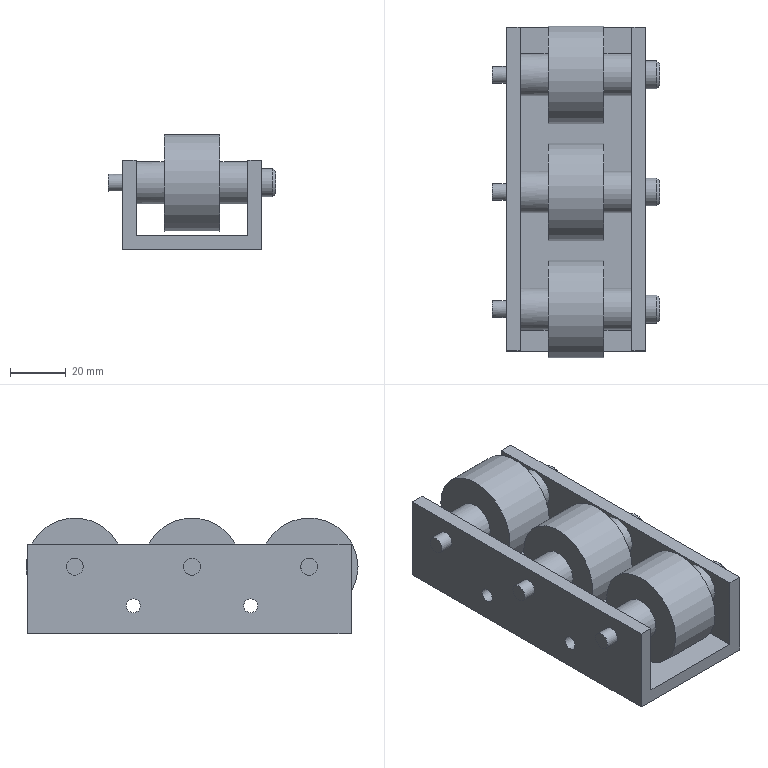Part | NX | features solid 2 | 1 solid | 44 faces | box 60 x 119 x 41.5 mm | volume 129815 mm3 | plane 22 | cylinder 19 | cone 3 | commonest cylinder face diameters 15 x6 5 x4 6 x3 10 x3 35 x3
STEP:
#1=CARTESIAN_POINT('',(215.,191.,-18.));
#2=VERTEX_POINT('',#1);
#3=CARTESIAN_POINT('',(215.,191.,-50.));
#4=VERTEX_POINT('',#3);
#5=CARTESIAN_POINT('',(215.,191.,-18.));
#6=DIRECTION('',(0.,0.,-1.));
#7=VECTOR('',#6,1000.);
#8=LINE('',#5,#7);
#9=EDGE_CURVE('',#2,#4,#8,.T.);
#10=ORIENTED_EDGE('',*,*,#9,.T.);
#11=CARTESIAN_POINT('',(165.,191.,-50.));
#12=VERTEX_POINT('',#11);
#13=CARTESIAN_POINT('',(215.,191.,-50.));
#14=DIRECTION('',(-1.,0.,0.));
#15=VECTOR('',#14,1000.);
#16=LINE('',#13,#15);
#17=EDGE_CURVE('',#4,#12,#16,.T.);
#18=ORIENTED_EDGE('',*,*,#17,.T.);
#19=CARTESIAN_POINT('',(165.,191.,-18.));
#20=VERTEX_POINT('',#19);
#21=CARTESIAN_POINT('',(165.,191.,-50.));
#22=DIRECTION('',(0.,0.,1.));
#23=VECTOR('',#22,1000.);
#24=LINE('',#21,#23);
#25=EDGE_CURVE('',#12,#20,#24,.T.);
#26=ORIENTED_EDGE('',*,*,#25,.T.);
#27=CARTESIAN_POINT('',(170.,191.,-18.));
#28=VERTEX_POINT('',#27);
#29=CARTESIAN_POINT('',(165.,191.,-18.));
#30=DIRECTION('',(1.,0.,0.));
#31=VECTOR('',#30,1000.);
#32=LINE('',#29,#31);
#33=EDGE_CURVE('',#20,#28,#32,.T.);
#34=ORIENTED_EDGE('',*,*,#33,.T.);
#35=CARTESIAN_POINT('',(170.,191.,-45.));
#36=VERTEX_POINT('',#35);
#37=CARTESIAN_POINT('',(170.,191.,-50.));
#38=DIRECTION('',(0.,0.,1.));
#39=VECTOR('',#38,1000.);
#40=LINE('',#37,#39);
#41=EDGE_CURVE('',#36,#28,#40,.T.);
#42=ORIENTED_EDGE('',*,*,#41,.F.);
#43=CARTESIAN_POINT('',(210.,191.,-45.));
#44=VERTEX_POINT('',#43);
#45=CARTESIAN_POINT('',(215.,191.,-45.));
#46=DIRECTION('',(-1.,0.,0.));
#47=VECTOR('',#46,1000.);
#48=LINE('',#45,#47);
#49=EDGE_CURVE('',#44,#36,#48,.T.);
#50=ORIENTED_EDGE('',*,*,#49,.F.);
#51=CARTESIAN_POINT('',(210.,191.,-18.));
#52=VERTEX_POINT('',#51);
#53=CARTESIAN_POINT('',(210.,191.,-18.));
#54=DIRECTION('',(0.,0.,-1.));
#55=VECTOR('',#54,1000.);
#56=LINE('',#53,#55);
#57=EDGE_CURVE('',#52,#44,#56,.T.);
#58=ORIENTED_EDGE('',*,*,#57,.F.);
#59=CARTESIAN_POINT('',(215.,191.,-18.));
#60=DIRECTION('',(-1.,0.,0.));
#61=VECTOR('',#60,1000.);
#62=LINE('',#59,#61);
#63=EDGE_CURVE('',#52,#2,#62,.F.);
#64=ORIENTED_EDGE('',*,*,#63,.T.);
#65=EDGE_LOOP('',(#10,#18,#26,#34,#42,#50,#58,#64));
#66=FACE_BOUND('',#65,.T.);
#67=CARTESIAN_POINT('',(190.,191.,-34.));
#68=DIRECTION('',(0.,1.,0.));
#69=DIRECTION('',(0.,0.,1.));
#70=AXIS2_PLACEMENT_3D('',#67,#68,#69);
#71=PLANE('',#70);
#72=ADVANCED_FACE('',(#66),#71,.T.);
#73=CARTESIAN_POINT('',(220.,174.,-22.));
#74=VERTEX_POINT('',#73);
#75=CARTESIAN_POINT('',(220.,174.,-26.));
#76=DIRECTION('',(1.,0.,0.));
#77=DIRECTION('',(0.,0.,1.));
#78=AXIS2_PLACEMENT_3D('',#75,#76,#77);
#79=CIRCLE('',#78,4.);
#80=EDGE_CURVE('',#74,#74,#79,.F.);
#81=ORIENTED_EDGE('',*,*,#80,.F.);
#82=EDGE_LOOP('',(#81));
#83=FACE_BOUND('',#82,.T.);
#84=CARTESIAN_POINT('',(220.,174.,-26.));
#85=DIRECTION('',(-1.,0.,0.));
#86=DIRECTION('',(0.,0.,1.));
#87=AXIS2_PLACEMENT_3D('',#84,#85,#86);
#88=PLANE('',#87);
#89=ADVANCED_FACE('',(#83),#88,.F.);
#90=CARTESIAN_POINT('',(220.,132.,-22.));
#91=VERTEX_POINT('',#90);
#92=CARTESIAN_POINT('',(220.,132.,-26.));
#93=DIRECTION('',(1.,0.,0.));
#94=DIRECTION('',(0.,0.,1.));
#95=AXIS2_PLACEMENT_3D('',#92,#93,#94);
#96=CIRCLE('',#95,4.);
#97=EDGE_CURVE('',#91,#91,#96,.F.);
#98=ORIENTED_EDGE('',*,*,#97,.F.);
#99=EDGE_LOOP('',(#98));
#100=FACE_BOUND('',#99,.T.);
#101=CARTESIAN_POINT('',(220.,132.,-26.));
#102=DIRECTION('',(-1.,0.,0.));
#103=DIRECTION('',(0.,0.,1.));
#104=AXIS2_PLACEMENT_3D('',#101,#102,#103);
#105=PLANE('',#104);
#106=ADVANCED_FACE('',(#100),#105,.F.);
#107=CARTESIAN_POINT('',(220.,90.,-22.));
#108=VERTEX_POINT('',#107);
#109=CARTESIAN_POINT('',(220.,90.,-26.));
#110=DIRECTION('',(1.,0.,0.));
#111=DIRECTION('',(0.,0.,1.));
#112=AXIS2_PLACEMENT_3D('',#109,#110,#111);
#113=CIRCLE('',#112,4.);
#114=EDGE_CURVE('',#108,#108,#113,.F.);
#115=ORIENTED_EDGE('',*,*,#114,.F.);
#116=EDGE_LOOP('',(#115));
#117=FACE_BOUND('',#116,.T.);
#118=CARTESIAN_POINT('',(220.,90.,-26.));
#119=DIRECTION('',(-1.,0.,0.));
#120=DIRECTION('',(0.,0.,1.));
#121=AXIS2_PLACEMENT_3D('',#118,#119,#120);
#122=PLANE('',#121);
#123=ADVANCED_FACE('',(#117),#122,.F.);
#124=CARTESIAN_POINT('',(180.,114.5,-26.));
#125=VERTEX_POINT('',#124);
#126=CARTESIAN_POINT('',(180.,132.,-26.));
#127=DIRECTION('',(1.,0.,0.));
#128=DIRECTION('',(0.,-1.,0.));
#129=AXIS2_PLACEMENT_3D('',#126,#127,#128);
#130=CIRCLE('',#129,17.5);
#131=EDGE_CURVE('',#125,#125,#130,.T.);
#132=ORIENTED_EDGE('',*,*,#131,.T.);
#133=EDGE_LOOP('',(#132));
#134=FACE_BOUND('',#133,.T.);
#135=CARTESIAN_POINT('',(200.,114.5,-26.));
#136=VERTEX_POINT('',#135);
#137=CARTESIAN_POINT('',(200.,132.,-26.));
#138=DIRECTION('',(1.,0.,0.));
#139=DIRECTION('',(0.,-1.,0.));
#140=AXIS2_PLACEMENT_3D('',#137,#138,#139);
#141=CIRCLE('',#140,17.5);
#142=EDGE_CURVE('',#136,#136,#141,.T.);
#143=ORIENTED_EDGE('',*,*,#142,.F.);
#144=EDGE_LOOP('',(#143));
#145=FACE_BOUND('',#144,.T.);
#146=CARTESIAN_POINT('',(180.,132.,-26.));
#147=DIRECTION('',(1.,0.,0.));
#148=DIRECTION('',(0.,0.,-1.));
#149=AXIS2_PLACEMENT_3D('',#146,#147,#148);
#150=CYLINDRICAL_SURFACE('',#149,17.5);
#151=ADVANCED_FACE('',(#134,#145),#150,.T.);
#152=CARTESIAN_POINT('',(200.,72.5,-26.));
#153=VERTEX_POINT('',#152);
#154=CARTESIAN_POINT('',(200.,90.,-26.));
#155=DIRECTION('',(1.,0.,0.));
#156=DIRECTION('',(0.,-1.,0.));
#157=AXIS2_PLACEMENT_3D('',#154,#155,#156);
#158=CIRCLE('',#157,17.5);
#159=EDGE_CURVE('',#153,#153,#158,.T.);
#160=ORIENTED_EDGE('',*,*,#159,.F.);
#161=EDGE_LOOP('',(#160));
#162=FACE_BOUND('',#161,.T.);
#163=CARTESIAN_POINT('',(180.,72.5,-26.));
#164=VERTEX_POINT('',#163);
#165=CARTESIAN_POINT('',(180.,90.,-26.));
#166=DIRECTION('',(1.,0.,0.));
#167=DIRECTION('',(0.,-1.,0.));
#168=AXIS2_PLACEMENT_3D('',#165,#166,#167);
#169=CIRCLE('',#168,17.5);
#170=EDGE_CURVE('',#164,#164,#169,.T.);
#171=ORIENTED_EDGE('',*,*,#170,.T.);
#172=EDGE_LOOP('',(#171));
#173=FACE_BOUND('',#172,.T.);
#174=CARTESIAN_POINT('',(180.,90.,-26.));
#175=DIRECTION('',(1.,0.,0.));
#176=DIRECTION('',(0.,0.,-1.));
#177=AXIS2_PLACEMENT_3D('',#174,#175,#176);
#178=CYLINDRICAL_SURFACE('',#177,17.5);
#179=ADVANCED_FACE('',(#162,#173),#178,.T.);
#180=ORIENTED_EDGE('',*,*,#80,.T.);
#181=EDGE_LOOP('',(#180));
#182=FACE_BOUND('',#181,.T.);
#183=CARTESIAN_POINT('',(219.,174.,-21.));
#184=VERTEX_POINT('',#183);
#185=CARTESIAN_POINT('',(219.,174.,-26.));
#186=DIRECTION('',(1.,0.,0.));
#187=DIRECTION('',(0.,0.,1.));
#188=AXIS2_PLACEMENT_3D('',#185,#186,#187);
#189=CIRCLE('',#188,5.);
#190=EDGE_CURVE('',#184,#184,#189,.T.);
#191=ORIENTED_EDGE('',*,*,#190,.T.);
#192=EDGE_LOOP('',(#191));
#193=FACE_BOUND('',#192,.T.);
#194=CARTESIAN_POINT('',(219.,174.,-26.));
#195=DIRECTION('',(-1.,0.,0.));
#196=DIRECTION('',(0.,0.,1.));
#197=AXIS2_PLACEMENT_3D('',#194,#195,#196);
#198=CONICAL_SURFACE('',#197,5.,0.7854);
#199=ADVANCED_FACE('',(#182,#193),#198,.T.);
#200=ORIENTED_EDGE('',*,*,#97,.T.);
#201=EDGE_LOOP('',(#200));
#202=FACE_BOUND('',#201,.T.);
#203=CARTESIAN_POINT('',(219.,132.,-21.));
#204=VERTEX_POINT('',#203);
#205=CARTESIAN_POINT('',(219.,132.,-26.));
#206=DIRECTION('',(1.,0.,0.));
#207=DIRECTION('',(0.,0.,1.));
#208=AXIS2_PLACEMENT_3D('',#205,#206,#207);
#209=CIRCLE('',#208,5.);
#210=EDGE_CURVE('',#204,#204,#209,.T.);
#211=ORIENTED_EDGE('',*,*,#210,.T.);
#212=EDGE_LOOP('',(#211));
#213=FACE_BOUND('',#212,.T.);
#214=CARTESIAN_POINT('',(219.,132.,-26.));
#215=DIRECTION('',(-1.,0.,0.));
#216=DIRECTION('',(0.,0.,1.));
#217=AXIS2_PLACEMENT_3D('',#214,#215,#216);
#218=CONICAL_SURFACE('',#217,5.,0.7854);
#219=ADVANCED_FACE('',(#202,#213),#218,.T.);
#220=ORIENTED_EDGE('',*,*,#114,.T.);
#221=EDGE_LOOP('',(#220));
#222=FACE_BOUND('',#221,.T.);
#223=CARTESIAN_POINT('',(219.,90.,-21.));
#224=VERTEX_POINT('',#223);
#225=CARTESIAN_POINT('',(219.,90.,-26.));
#226=DIRECTION('',(1.,0.,0.));
#227=DIRECTION('',(0.,0.,1.));
#228=AXIS2_PLACEMENT_3D('',#225,#226,#227);
#229=CIRCLE('',#228,5.);
#230=EDGE_CURVE('',#224,#224,#229,.T.);
#231=ORIENTED_EDGE('',*,*,#230,.T.);
#232=EDGE_LOOP('',(#231));
#233=FACE_BOUND('',#232,.T.);
#234=CARTESIAN_POINT('',(219.,90.,-26.));
#235=DIRECTION('',(-1.,0.,0.));
#236=DIRECTION('',(0.,0.,1.));
#237=AXIS2_PLACEMENT_3D('',#234,#235,#236);
#238=CONICAL_SURFACE('',#237,5.,0.7854);
#239=ADVANCED_FACE('',(#222,#233),#238,.T.);
#240=CARTESIAN_POINT('',(160.,129.,-26.));
#241=VERTEX_POINT('',#240);
#242=CARTESIAN_POINT('',(160.,132.,-26.));
#243=DIRECTION('',(1.,0.,0.));
#244=DIRECTION('',(0.,-1.,0.));
#245=AXIS2_PLACEMENT_3D('',#242,#243,#244);
#246=CIRCLE('',#245,3.);
#247=EDGE_CURVE('',#241,#241,#246,.T.);
#248=ORIENTED_EDGE('',*,*,#247,.F.);
#249=EDGE_LOOP('',(#248));
#250=FACE_BOUND('',#249,.T.);
#251=CARTESIAN_POINT('',(160.,132.,-26.));
#252=DIRECTION('',(-1.,0.,0.));
#253=DIRECTION('',(0.,0.,1.));
#254=AXIS2_PLACEMENT_3D('',#251,#252,#253);
#255=PLANE('',#254);
#256=ADVANCED_FACE('',(#250),#255,.T.);
#257=CARTESIAN_POINT('',(160.,171.,-26.));
#258=VERTEX_POINT('',#257);
#259=CARTESIAN_POINT('',(160.,174.,-26.));
#260=DIRECTION('',(1.,0.,0.));
#261=DIRECTION('',(0.,-1.,0.));
#262=AXIS2_PLACEMENT_3D('',#259,#260,#261);
#263=CIRCLE('',#262,3.);
#264=EDGE_CURVE('',#258,#258,#263,.T.);
#265=ORIENTED_EDGE('',*,*,#264,.F.);
#266=EDGE_LOOP('',(#265));
#267=FACE_BOUND('',#266,.T.);
#268=CARTESIAN_POINT('',(160.,174.,-26.));
#269=DIRECTION('',(-1.,0.,0.));
#270=DIRECTION('',(0.,0.,1.));
#271=AXIS2_PLACEMENT_3D('',#268,#269,#270);
#272=PLANE('',#271);
#273=ADVANCED_FACE('',(#267),#272,.T.);
#274=CARTESIAN_POINT('',(160.,87.,-26.));
#275=VERTEX_POINT('',#274);
#276=CARTESIAN_POINT('',(160.,90.,-26.));
#277=DIRECTION('',(1.,0.,0.));
#278=DIRECTION('',(0.,-1.,0.));
#279=AXIS2_PLACEMENT_3D('',#276,#277,#278);
#280=CIRCLE('',#279,3.);
#281=EDGE_CURVE('',#275,#275,#280,.T.);
#282=ORIENTED_EDGE('',*,*,#281,.F.);
#283=EDGE_LOOP('',(#282));
#284=FACE_BOUND('',#283,.T.);
#285=CARTESIAN_POINT('',(160.,90.,-26.));
#286=DIRECTION('',(-1.,0.,0.));
#287=DIRECTION('',(0.,0.,1.));
#288=AXIS2_PLACEMENT_3D('',#285,#286,#287);
#289=PLANE('',#288);
#290=ADVANCED_FACE('',(#284),#289,.T.);
#291=CARTESIAN_POINT('',(200.,124.5,-26.));
#292=VERTEX_POINT('',#291);
#293=CARTESIAN_POINT('',(200.,132.,-26.));
#294=DIRECTION('',(1.,0.,0.));
#295=DIRECTION('',(0.,-1.,0.));
#296=AXIS2_PLACEMENT_3D('',#293,#294,#295);
#297=CIRCLE('',#296,7.5);
#298=EDGE_CURVE('',#292,#292,#297,.T.);
#299=ORIENTED_EDGE('',*,*,#298,.F.);
#300=EDGE_LOOP('',(#299));
#301=FACE_BOUND('',#300,.T.);
#302=ORIENTED_EDGE('',*,*,#142,.T.);
#303=EDGE_LOOP('',(#302));
#304=FACE_BOUND('',#303,.T.);
#305=CARTESIAN_POINT('',(200.,132.,-26.));
#306=DIRECTION('',(-1.,0.,0.));
#307=DIRECTION('',(0.,0.,1.));
#308=AXIS2_PLACEMENT_3D('',#305,#306,#307);
#309=PLANE('',#308);
#310=ADVANCED_FACE('',(#301,#304),#309,.F.);
#311=CARTESIAN_POINT('',(200.,82.5,-26.));
#312=VERTEX_POINT('',#311);
#313=CARTESIAN_POINT('',(200.,90.,-26.));
#314=DIRECTION('',(1.,0.,0.));
#315=DIRECTION('',(0.,-1.,0.));
#316=AXIS2_PLACEMENT_3D('',#313,#314,#315);
#317=CIRCLE('',#316,7.5);
#318=EDGE_CURVE('',#312,#312,#317,.T.);
#319=ORIENTED_EDGE('',*,*,#318,.F.);
#320=EDGE_LOOP('',(#319));
#321=FACE_BOUND('',#320,.T.);
#322=ORIENTED_EDGE('',*,*,#159,.T.);
#323=EDGE_LOOP('',(#322));
#324=FACE_BOUND('',#323,.T.);
#325=CARTESIAN_POINT('',(200.,90.,-26.));
#326=DIRECTION('',(-1.,0.,0.));
#327=DIRECTION('',(0.,0.,1.));
#328=AXIS2_PLACEMENT_3D('',#325,#326,#327);
#329=PLANE('',#328);
#330=ADVANCED_FACE('',(#321,#324),#329,.F.);
#331=ORIENTED_EDGE('',*,*,#131,.F.);
#332=EDGE_LOOP('',(#331));
#333=FACE_BOUND('',#332,.T.);
#334=CARTESIAN_POINT('',(180.,124.5,-26.));
#335=VERTEX_POINT('',#334);
#336=CARTESIAN_POINT('',(180.,132.,-26.));
#337=DIRECTION('',(1.,0.,0.));
#338=DIRECTION('',(0.,-1.,0.));
#339=AXIS2_PLACEMENT_3D('',#336,#337,#338);
#340=CIRCLE('',#339,7.5);
#341=EDGE_CURVE('',#335,#335,#340,.T.);
#342=ORIENTED_EDGE('',*,*,#341,.T.);
#343=EDGE_LOOP('',(#342));
#344=FACE_BOUND('',#343,.T.);
#345=CARTESIAN_POINT('',(180.,132.,-26.));
#346=DIRECTION('',(-1.,0.,0.));
#347=DIRECTION('',(0.,0.,1.));
#348=AXIS2_PLACEMENT_3D('',#345,#346,#347);
#349=PLANE('',#348);
#350=ADVANCED_FACE('',(#333,#344),#349,.T.);
#351=CARTESIAN_POINT('',(180.,82.5,-26.));
#352=VERTEX_POINT('',#351);
#353=CARTESIAN_POINT('',(180.,90.,-26.));
#354=DIRECTION('',(1.,0.,0.));
#355=DIRECTION('',(0.,-1.,0.));
#356=AXIS2_PLACEMENT_3D('',#353,#354,#355);
#357=CIRCLE('',#356,7.5);
#358=EDGE_CURVE('',#352,#352,#357,.T.);
#359=ORIENTED_EDGE('',*,*,#358,.T.);
#360=EDGE_LOOP('',(#359));
#361=FACE_BOUND('',#360,.T.);
#362=ORIENTED_EDGE('',*,*,#170,.F.);
#363=EDGE_LOOP('',(#362));
#364=FACE_BOUND('',#363,.T.);
#365=CARTESIAN_POINT('',(180.,90.,-26.));
#366=DIRECTION('',(-1.,0.,0.));
#367=DIRECTION('',(0.,0.,1.));
#368=AXIS2_PLACEMENT_3D('',#365,#366,#367);
#369=PLANE('',#368);
#370=ADVANCED_FACE('',(#361,#364),#369,.T.);
#371=ORIENTED_EDGE('',*,*,#190,.F.);
#372=EDGE_LOOP('',(#371));
#373=FACE_BOUND('',#372,.T.);
#374=CARTESIAN_POINT('',(215.,174.,-31.));
#375=VERTEX_POINT('',#374);
#376=CARTESIAN_POINT('',(215.,174.,-26.));
#377=DIRECTION('',(-1.,0.,0.));
#378=DIRECTION('',(0.,0.,-1.));
#379=AXIS2_PLACEMENT_3D('',#376,#377,#378);
#380=CIRCLE('',#379,5.);
#381=EDGE_CURVE('',#375,#375,#380,.T.);
#382=ORIENTED_EDGE('',*,*,#381,.F.);
#383=EDGE_LOOP('',(#382));
#384=FACE_BOUND('',#383,.T.);
#385=CARTESIAN_POINT('',(220.,174.,-26.));
#386=DIRECTION('',(-1.,0.,0.));
#387=DIRECTION('',(0.,0.,1.));
#388=AXIS2_PLACEMENT_3D('',#385,#386,#387);
#389=CYLINDRICAL_SURFACE('',#388,5.);
#390=ADVANCED_FACE('',(#373,#384),#389,.T.);
#391=ORIENTED_EDGE('',*,*,#210,.F.);
#392=EDGE_LOOP('',(#391));
#393=FACE_BOUND('',#392,.T.);
#394=CARTESIAN_POINT('',(215.,132.,-31.));
#395=VERTEX_POINT('',#394);
#396=CARTESIAN_POINT('',(215.,132.,-26.));
#397=DIRECTION('',(-1.,0.,0.));
#398=DIRECTION('',(0.,0.,-1.));
#399=AXIS2_PLACEMENT_3D('',#396,#397,#398);
#400=CIRCLE('',#399,5.);
#401=EDGE_CURVE('',#395,#395,#400,.T.);
#402=ORIENTED_EDGE('',*,*,#401,.F.);
#403=EDGE_LOOP('',(#402));
#404=FACE_BOUND('',#403,.T.);
#405=CARTESIAN_POINT('',(220.,132.,-26.));
#406=DIRECTION('',(-1.,0.,0.));
#407=DIRECTION('',(0.,0.,1.));
#408=AXIS2_PLACEMENT_3D('',#405,#406,#407);
#409=CYLINDRICAL_SURFACE('',#408,5.);
#410=ADVANCED_FACE('',(#393,#404),#409,.T.);
#411=ORIENTED_EDGE('',*,*,#230,.F.);
#412=EDGE_LOOP('',(#411));
#413=FACE_BOUND('',#412,.T.);
#414=CARTESIAN_POINT('',(215.,90.,-31.));
#415=VERTEX_POINT('',#414);
#416=CARTESIAN_POINT('',(215.,90.,-26.));
#417=DIRECTION('',(-1.,0.,0.));
#418=DIRECTION('',(0.,0.,-1.));
#419=AXIS2_PLACEMENT_3D('',#416,#417,#418);
#420=CIRCLE('',#419,5.);
#421=EDGE_CURVE('',#415,#415,#420,.T.);
#422=ORIENTED_EDGE('',*,*,#421,.F.);
#423=EDGE_LOOP('',(#422));
#424=FACE_BOUND('',#423,.T.);
#425=CARTESIAN_POINT('',(220.,90.,-26.));
#426=DIRECTION('',(-1.,0.,0.));
#427=DIRECTION('',(0.,0.,1.));
#428=AXIS2_PLACEMENT_3D('',#425,#426,#427);
#429=CYLINDRICAL_SURFACE('',#428,5.);
#430=ADVANCED_FACE('',(#413,#424),#429,.T.);
#431=CARTESIAN_POINT('',(165.,132.,-23.));
#432=VERTEX_POINT('',#431);
#433=CARTESIAN_POINT('',(165.,132.,-26.));
#434=DIRECTION('',(1.,0.,0.));
#435=DIRECTION('',(0.,0.,1.));
#436=AXIS2_PLACEMENT_3D('',#433,#434,#435);
#437=CIRCLE('',#436,3.);
#438=EDGE_CURVE('',#432,#432,#437,.F.);
#439=ORIENTED_EDGE('',*,*,#438,.T.);
#440=EDGE_LOOP('',(#439));
#441=FACE_BOUND('',#440,.T.);
#442=ORIENTED_EDGE('',*,*,#247,.T.);
#443=EDGE_LOOP('',(#442));
#444=FACE_BOUND('',#443,.T.);
#445=CARTESIAN_POINT('',(160.,132.,-26.));
#446=DIRECTION('',(1.,0.,0.));
#447=DIRECTION('',(0.,0.,-1.));
#448=AXIS2_PLACEMENT_3D('',#445,#446,#447);
#449=CYLINDRICAL_SURFACE('',#448,3.);
#450=ADVANCED_FACE('',(#441,#444),#449,.T.);
#451=CARTESIAN_POINT('',(165.,174.,-23.));
#452=VERTEX_POINT('',#451);
#453=CARTESIAN_POINT('',(165.,174.,-26.));
#454=DIRECTION('',(1.,0.,0.));
#455=DIRECTION('',(0.,0.,1.));
#456=AXIS2_PLACEMENT_3D('',#453,#454,#455);
#457=CIRCLE('',#456,3.);
#458=EDGE_CURVE('',#452,#452,#457,.F.);
#459=ORIENTED_EDGE('',*,*,#458,.T.);
#460=EDGE_LOOP('',(#459));
#461=FACE_BOUND('',#460,.T.);
#462=ORIENTED_EDGE('',*,*,#264,.T.);
#463=EDGE_LOOP('',(#462));
#464=FACE_BOUND('',#463,.T.);
#465=CARTESIAN_POINT('',(160.,174.,-26.));
#466=DIRECTION('',(1.,0.,0.));
#467=DIRECTION('',(0.,0.,-1.));
#468=AXIS2_PLACEMENT_3D('',#465,#466,#467);
#469=CYLINDRICAL_SURFACE('',#468,3.);
#470=ADVANCED_FACE('',(#461,#464),#469,.T.);
#471=CARTESIAN_POINT('',(165.,90.,-23.));
#472=VERTEX_POINT('',#471);
#473=CARTESIAN_POINT('',(165.,90.,-26.));
#474=DIRECTION('',(1.,0.,0.));
#475=DIRECTION('',(0.,0.,1.));
#476=AXIS2_PLACEMENT_3D('',#473,#474,#475);
#477=CIRCLE('',#476,3.);
#478=EDGE_CURVE('',#472,#472,#477,.F.);
#479=ORIENTED_EDGE('',*,*,#478,.T.);
#480=EDGE_LOOP('',(#479));
#481=FACE_BOUND('',#480,.T.);
#482=ORIENTED_EDGE('',*,*,#281,.T.);
#483=EDGE_LOOP('',(#482));
#484=FACE_BOUND('',#483,.T.);
#485=CARTESIAN_POINT('',(160.,90.,-26.));
#486=DIRECTION('',(1.,0.,0.));
#487=DIRECTION('',(0.,0.,-1.));
#488=AXIS2_PLACEMENT_3D('',#485,#486,#487);
#489=CYLINDRICAL_SURFACE('',#488,3.);
#490=ADVANCED_FACE('',(#481,#484),#489,.T.);
#491=CARTESIAN_POINT('',(215.,111.,-42.5));
#492=VERTEX_POINT('',#491);
#493=CARTESIAN_POINT('',(215.,111.,-40.));
#494=DIRECTION('',(-1.,0.,0.));
#495=DIRECTION('',(0.,0.,-1.));
#496=AXIS2_PLACEMENT_3D('',#493,#494,#495);
#497=CIRCLE('',#496,2.5);
#498=EDGE_CURVE('',#492,#492,#497,.F.);
#499=ORIENTED_EDGE('',*,*,#498,.T.);
#500=EDGE_LOOP('',(#499));
#501=FACE_BOUND('',#500,.T.);
#502=CARTESIAN_POINT('',(210.,111.,-42.5));
#503=VERTEX_POINT('',#502);
#504=CARTESIAN_POINT('',(210.,111.,-40.));
#505=DIRECTION('',(-1.,0.,0.));
#506=DIRECTION('',(0.,0.,-1.));
#507=AXIS2_PLACEMENT_3D('',#504,#505,#506);
#508=CIRCLE('',#507,2.5);
#509=EDGE_CURVE('',#503,#503,#508,.F.);
#510=ORIENTED_EDGE('',*,*,#509,.F.);
#511=EDGE_LOOP('',(#510));
#512=FACE_BOUND('',#511,.T.);
#513=CARTESIAN_POINT('',(160.,111.,-40.));
#514=DIRECTION('',(1.,0.,0.));
#515=DIRECTION('',(0.,0.,-1.));
#516=AXIS2_PLACEMENT_3D('',#513,#514,#515);
#517=CYLINDRICAL_SURFACE('',#516,2.5);
#518=ADVANCED_FACE('',(#501,#512),#517,.F.);
#519=CARTESIAN_POINT('',(210.,124.5,-26.));
#520=VERTEX_POINT('',#519);
#521=CARTESIAN_POINT('',(210.,132.,-26.));
#522=DIRECTION('',(1.,0.,0.));
#523=DIRECTION('',(0.,-1.,0.));
#524=AXIS2_PLACEMENT_3D('',#521,#522,#523);
#525=CIRCLE('',#524,7.5);
#526=EDGE_CURVE('',#520,#520,#525,.T.);
#527=ORIENTED_EDGE('',*,*,#526,.F.);
#528=EDGE_LOOP('',(#527));
#529=FACE_BOUND('',#528,.T.);
#530=ORIENTED_EDGE('',*,*,#298,.T.);
#531=EDGE_LOOP('',(#530));
#532=FACE_BOUND('',#531,.T.);
#533=CARTESIAN_POINT('',(210.,132.,-26.));
#534=DIRECTION('',(-1.,0.,0.));
#535=DIRECTION('',(0.,0.,1.));
#536=AXIS2_PLACEMENT_3D('',#533,#534,#535);
#537=CYLINDRICAL_SURFACE('',#536,7.5);
#538=ADVANCED_FACE('',(#529,#532),#537,.T.);
#539=CARTESIAN_POINT('',(210.,82.5,-26.));
#540=VERTEX_POINT('',#539);
#541=CARTESIAN_POINT('',(210.,90.,-26.));
#542=DIRECTION('',(1.,0.,0.));
#543=DIRECTION('',(0.,-1.,0.));
#544=AXIS2_PLACEMENT_3D('',#541,#542,#543);
#545=CIRCLE('',#544,7.5);
#546=EDGE_CURVE('',#540,#540,#545,.T.);
#547=ORIENTED_EDGE('',*,*,#546,.F.);
#548=EDGE_LOOP('',(#547));
#549=FACE_BOUND('',#548,.T.);
#550=ORIENTED_EDGE('',*,*,#318,.T.);
#551=EDGE_LOOP('',(#550));
#552=FACE_BOUND('',#551,.T.);
#553=CARTESIAN_POINT('',(210.,90.,-26.));
#554=DIRECTION('',(-1.,0.,0.));
#555=DIRECTION('',(0.,0.,1.));
#556=AXIS2_PLACEMENT_3D('',#553,#554,#555);
#557=CYLINDRICAL_SURFACE('',#556,7.5);
#558=ADVANCED_FACE('',(#549,#552),#557,.T.);
#559=CARTESIAN_POINT('',(215.,153.,-42.5));
#560=VERTEX_POINT('',#559);
#561=CARTESIAN_POINT('',(215.,153.,-40.));
#562=DIRECTION('',(-1.,0.,0.));
#563=DIRECTION('',(0.,0.,-1.));
#564=AXIS2_PLACEMENT_3D('',#561,#562,#563);
#565=CIRCLE('',#564,2.5);
#566=EDGE_CURVE('',#560,#560,#565,.F.);
#567=ORIENTED_EDGE('',*,*,#566,.T.);
#568=EDGE_LOOP('',(#567));
#569=FACE_BOUND('',#568,.T.);
#570=CARTESIAN_POINT('',(210.,153.,-42.5));
#571=VERTEX_POINT('',#570);
#572=CARTESIAN_POINT('',(210.,153.,-40.));
#573=DIRECTION('',(-1.,0.,0.));
#574=DIRECTION('',(0.,0.,-1.));
#575=AXIS2_PLACEMENT_3D('',#572,#573,#574);
#576=CIRCLE('',#575,2.5);
#577=EDGE_CURVE('',#571,#571,#576,.F.);
#578=ORIENTED_EDGE('',*,*,#577,.F.);
#579=EDGE_LOOP('',(#578));
#580=FACE_BOUND('',#579,.T.);
#581=CARTESIAN_POINT('',(160.,153.,-40.));
#582=DIRECTION('',(1.,0.,0.));
#583=DIRECTION('',(0.,0.,-1.));
#584=AXIS2_PLACEMENT_3D('',#581,#582,#583);
#585=CYLINDRICAL_SURFACE('',#584,2.5);
#586=ADVANCED_FACE('',(#569,#580),#585,.F.);
#587=CARTESIAN_POINT('',(170.,75.,-18.));
#588=VERTEX_POINT('',#587);
#589=CARTESIAN_POINT('',(170.,75.,-45.));
#590=VERTEX_POINT('',#589);
#591=CARTESIAN_POINT('',(170.,75.,-50.));
#592=DIRECTION('',(0.,0.,-1.));
#593=VECTOR('',#592,1000.);
#594=LINE('',#591,#593);
#595=EDGE_CURVE('',#588,#590,#594,.T.);
#596=ORIENTED_EDGE('',*,*,#595,.F.);
#597=CARTESIAN_POINT('',(165.,75.,-18.));
#598=VERTEX_POINT('',#597);
#599=CARTESIAN_POINT('',(165.,75.,-18.));
#600=DIRECTION('',(-1.,0.,0.));
#601=VECTOR('',#600,1000.);
#602=LINE('',#599,#601);
#603=EDGE_CURVE('',#588,#598,#602,.T.);
#604=ORIENTED_EDGE('',*,*,#603,.T.);
#605=CARTESIAN_POINT('',(165.,75.,-50.));
#606=VERTEX_POINT('',#605);
#607=CARTESIAN_POINT('',(165.,75.,-50.));
#608=DIRECTION('',(0.,0.,-1.));
#609=VECTOR('',#608,1000.);
#610=LINE('',#607,#609);
#611=EDGE_CURVE('',#598,#606,#610,.T.);
#612=ORIENTED_EDGE('',*,*,#611,.T.);
#613=CARTESIAN_POINT('',(215.,75.,-50.));
#614=VERTEX_POINT('',#613);
#615=CARTESIAN_POINT('',(215.,75.,-50.));
#616=DIRECTION('',(1.,0.,0.));
#617=VECTOR('',#616,1000.);
#618=LINE('',#615,#617);
#619=EDGE_CURVE('',#606,#614,#618,.T.);
#620=ORIENTED_EDGE('',*,*,#619,.T.);
#621=CARTESIAN_POINT('',(215.,75.,-18.));
#622=VERTEX_POINT('',#621);
#623=CARTESIAN_POINT('',(215.,75.,-18.));
#624=DIRECTION('',(0.,0.,1.));
#625=VECTOR('',#624,1000.);
#626=LINE('',#623,#625);
#627=EDGE_CURVE('',#614,#622,#626,.T.);
#628=ORIENTED_EDGE('',*,*,#627,.T.);
#629=CARTESIAN_POINT('',(210.,75.,-18.));
#630=VERTEX_POINT('',#629);
#631=CARTESIAN_POINT('',(215.,75.,-18.));
#632=DIRECTION('',(1.,0.,0.));
#633=VECTOR('',#632,1000.);
#634=LINE('',#631,#633);
#635=EDGE_CURVE('',#622,#630,#634,.F.);
#636=ORIENTED_EDGE('',*,*,#635,.T.);
#637=CARTESIAN_POINT('',(210.,75.,-45.));
#638=VERTEX_POINT('',#637);
#639=CARTESIAN_POINT('',(210.,75.,-18.));
#640=DIRECTION('',(0.,0.,1.));
#641=VECTOR('',#640,1000.);
#642=LINE('',#639,#641);
#643=EDGE_CURVE('',#638,#630,#642,.T.);
#644=ORIENTED_EDGE('',*,*,#643,.F.);
#645=CARTESIAN_POINT('',(215.,75.,-45.));
#646=DIRECTION('',(1.,0.,0.));
#647=VECTOR('',#646,1000.);
#648=LINE('',#645,#647);
#649=EDGE_CURVE('',#590,#638,#648,.T.);
#650=ORIENTED_EDGE('',*,*,#649,.F.);
#651=EDGE_LOOP('',(#596,#604,#612,#620,#628,#636,#644,#650));
#652=FACE_BOUND('',#651,.T.);
#653=CARTESIAN_POINT('',(190.,75.,-34.));
#654=DIRECTION('',(0.,-1.,0.));
#655=DIRECTION('',(0.,0.,-1.));
#656=AXIS2_PLACEMENT_3D('',#653,#654,#655);
#657=PLANE('',#656);
#658=ADVANCED_FACE('',(#652),#657,.T.);
#659=CARTESIAN_POINT('',(165.,111.,-37.5));
#660=VERTEX_POINT('',#659);
#661=CARTESIAN_POINT('',(165.,111.,-40.));
#662=DIRECTION('',(1.,0.,0.));
#663=DIRECTION('',(0.,0.,1.));
#664=AXIS2_PLACEMENT_3D('',#661,#662,#663);
#665=CIRCLE('',#664,2.5);
#666=EDGE_CURVE('',#660,#660,#665,.F.);
#667=ORIENTED_EDGE('',*,*,#666,.T.);
#668=EDGE_LOOP('',(#667));
#669=FACE_BOUND('',#668,.T.);
#670=CARTESIAN_POINT('',(170.,111.,-37.5));
#671=VERTEX_POINT('',#670);
#672=CARTESIAN_POINT('',(170.,111.,-40.));
#673=DIRECTION('',(1.,0.,0.));
#674=DIRECTION('',(0.,0.,1.));
#675=AXIS2_PLACEMENT_3D('',#672,#673,#674);
#676=CIRCLE('',#675,2.5);
#677=EDGE_CURVE('',#671,#671,#676,.F.);
#678=ORIENTED_EDGE('',*,*,#677,.F.);
#679=EDGE_LOOP('',(#678));
#680=FACE_BOUND('',#679,.T.);
#681=CARTESIAN_POINT('',(160.,111.,-40.));
#682=DIRECTION('',(1.,0.,0.));
#683=DIRECTION('',(0.,0.,-1.));
#684=AXIS2_PLACEMENT_3D('',#681,#682,#683);
#685=CYLINDRICAL_SURFACE('',#684,2.5);
#686=ADVANCED_FACE('',(#669,#680),#685,.F.);
#687=CARTESIAN_POINT('',(170.,132.,-18.5));
#688=VERTEX_POINT('',#687);
#689=CARTESIAN_POINT('',(170.,132.,-26.));
#690=DIRECTION('',(1.,0.,0.));
#691=DIRECTION('',(0.,0.,1.));
#692=AXIS2_PLACEMENT_3D('',#689,#690,#691);
#693=CIRCLE('',#692,7.5);
#694=EDGE_CURVE('',#688,#688,#693,.F.);
#695=ORIENTED_EDGE('',*,*,#694,.F.);
#696=EDGE_LOOP('',(#695));
#697=FACE_BOUND('',#696,.T.);
#698=ORIENTED_EDGE('',*,*,#341,.F.);
#699=EDGE_LOOP('',(#698));
#700=FACE_BOUND('',#699,.T.);
#701=CARTESIAN_POINT('',(170.,132.,-26.));
#702=DIRECTION('',(1.,0.,0.));
#703=DIRECTION('',(0.,0.,-1.));
#704=AXIS2_PLACEMENT_3D('',#701,#702,#703);
#705=CYLINDRICAL_SURFACE('',#704,7.5);
#706=ADVANCED_FACE('',(#697,#700),#705,.T.);
#707=CARTESIAN_POINT('',(170.,90.,-18.5));
#708=VERTEX_POINT('',#707);
#709=CARTESIAN_POINT('',(170.,90.,-26.));
#710=DIRECTION('',(1.,0.,0.));
#711=DIRECTION('',(0.,0.,1.));
#712=AXIS2_PLACEMENT_3D('',#709,#710,#711);
#713=CIRCLE('',#712,7.5);
#714=EDGE_CURVE('',#708,#708,#713,.F.);
#715=ORIENTED_EDGE('',*,*,#714,.F.);
#716=EDGE_LOOP('',(#715));
#717=FACE_BOUND('',#716,.T.);
#718=ORIENTED_EDGE('',*,*,#358,.F.);
#719=EDGE_LOOP('',(#718));
#720=FACE_BOUND('',#719,.T.);
#721=CARTESIAN_POINT('',(170.,90.,-26.));
#722=DIRECTION('',(1.,0.,0.));
#723=DIRECTION('',(0.,0.,-1.));
#724=AXIS2_PLACEMENT_3D('',#721,#722,#723);
#725=CYLINDRICAL_SURFACE('',#724,7.5);
#726=ADVANCED_FACE('',(#717,#720),#725,.T.);
#727=CARTESIAN_POINT('',(165.,153.,-37.5));
#728=VERTEX_POINT('',#727);
#729=CARTESIAN_POINT('',(165.,153.,-40.));
#730=DIRECTION('',(1.,0.,0.));
#731=DIRECTION('',(0.,0.,1.));
#732=AXIS2_PLACEMENT_3D('',#729,#730,#731);
#733=CIRCLE('',#732,2.5);
#734=EDGE_CURVE('',#728,#728,#733,.F.);
#735=ORIENTED_EDGE('',*,*,#734,.T.);
#736=EDGE_LOOP('',(#735));
#737=FACE_BOUND('',#736,.T.);
#738=CARTESIAN_POINT('',(170.,153.,-37.5));
#739=VERTEX_POINT('',#738);
#740=CARTESIAN_POINT('',(170.,153.,-40.));
#741=DIRECTION('',(1.,0.,0.));
#742=DIRECTION('',(0.,0.,1.));
#743=AXIS2_PLACEMENT_3D('',#740,#741,#742);
#744=CIRCLE('',#743,2.5);
#745=EDGE_CURVE('',#739,#739,#744,.F.);
#746=ORIENTED_EDGE('',*,*,#745,.F.);
#747=EDGE_LOOP('',(#746));
#748=FACE_BOUND('',#747,.T.);
#749=CARTESIAN_POINT('',(160.,153.,-40.));
#750=DIRECTION('',(1.,0.,0.));
#751=DIRECTION('',(0.,0.,-1.));
#752=AXIS2_PLACEMENT_3D('',#749,#750,#751);
#753=CYLINDRICAL_SURFACE('',#752,2.5);
#754=ADVANCED_FACE('',(#737,#748),#753,.F.);
#755=CARTESIAN_POINT('',(170.,174.,-18.5));
#756=VERTEX_POINT('',#755);
#757=CARTESIAN_POINT('',(170.,174.,-26.));
#758=DIRECTION('',(1.,0.,0.));
#759=DIRECTION('',(0.,0.,1.));
#760=AXIS2_PLACEMENT_3D('',#757,#758,#759);
#761=CIRCLE('',#760,7.5);
#762=EDGE_CURVE('',#756,#756,#761,.F.);
#763=ORIENTED_EDGE('',*,*,#762,.F.);
#764=EDGE_LOOP('',(#763));
#765=FACE_BOUND('',#764,.T.);
#766=CARTESIAN_POINT('',(180.,166.5,-26.));
#767=VERTEX_POINT('',#766);
#768=CARTESIAN_POINT('',(180.,174.,-26.));
#769=DIRECTION('',(1.,0.,0.));
#770=DIRECTION('',(0.,-1.,0.));
#771=AXIS2_PLACEMENT_3D('',#768,#769,#770);
#772=CIRCLE('',#771,7.5);
#773=EDGE_CURVE('',#767,#767,#772,.T.);
#774=ORIENTED_EDGE('',*,*,#773,.F.);
#775=EDGE_LOOP('',(#774));
#776=FACE_BOUND('',#775,.T.);
#777=CARTESIAN_POINT('',(170.,174.,-26.));
#778=DIRECTION('',(1.,0.,0.));
#779=DIRECTION('',(0.,0.,-1.));
#780=AXIS2_PLACEMENT_3D('',#777,#778,#779);
#781=CYLINDRICAL_SURFACE('',#780,7.5);
#782=ADVANCED_FACE('',(#765,#776),#781,.T.);
#783=ORIENTED_EDGE('',*,*,#745,.T.);
#784=EDGE_LOOP('',(#783));
#785=FACE_BOUND('',#784,.T.);
#786=ORIENTED_EDGE('',*,*,#714,.T.);
#787=EDGE_LOOP('',(#786));
#788=FACE_BOUND('',#787,.T.);
#789=ORIENTED_EDGE('',*,*,#762,.T.);
#790=EDGE_LOOP('',(#789));
#791=FACE_BOUND('',#790,.T.);
#792=ORIENTED_EDGE('',*,*,#694,.T.);
#793=EDGE_LOOP('',(#792));
#794=FACE_BOUND('',#793,.T.);
#795=ORIENTED_EDGE('',*,*,#677,.T.);
#796=EDGE_LOOP('',(#795));
#797=FACE_BOUND('',#796,.T.);
#798=ORIENTED_EDGE('',*,*,#41,.T.);
#799=CARTESIAN_POINT('',(170.,315.,-18.));
#800=DIRECTION('',(0.,-1.,0.));
#801=VECTOR('',#800,1000.);
#802=LINE('',#799,#801);
#803=EDGE_CURVE('',#28,#588,#802,.T.);
#804=ORIENTED_EDGE('',*,*,#803,.T.);
#805=ORIENTED_EDGE('',*,*,#595,.T.);
#806=CARTESIAN_POINT('',(170.,315.,-45.));
#807=DIRECTION('',(0.,-1.,0.));
#808=VECTOR('',#807,1000.);
#809=LINE('',#806,#808);
#810=EDGE_CURVE('',#36,#590,#809,.T.);
#811=ORIENTED_EDGE('',*,*,#810,.F.);
#812=EDGE_LOOP('',(#798,#804,#805,#811));
#813=FACE_BOUND('',#812,.T.);
#814=CARTESIAN_POINT('',(170.,315.,-50.));
#815=DIRECTION('',(-1.,0.,0.));
#816=DIRECTION('',(0.,0.,1.));
#817=AXIS2_PLACEMENT_3D('',#814,#815,#816);
#818=PLANE('',#817);
#819=ADVANCED_FACE('',(#785,#788,#791,#794,#797,#813),#818,.F.);
#820=ORIENTED_EDGE('',*,*,#577,.T.);
#821=EDGE_LOOP('',(#820));
#822=FACE_BOUND('',#821,.T.);
#823=ORIENTED_EDGE('',*,*,#546,.T.);
#824=EDGE_LOOP('',(#823));
#825=FACE_BOUND('',#824,.T.);
#826=ORIENTED_EDGE('',*,*,#526,.T.);
#827=EDGE_LOOP('',(#826));
#828=FACE_BOUND('',#827,.T.);
#829=CARTESIAN_POINT('',(210.,166.5,-26.));
#830=VERTEX_POINT('',#829);
#831=CARTESIAN_POINT('',(210.,174.,-26.));
#832=DIRECTION('',(1.,0.,0.));
#833=DIRECTION('',(0.,-1.,0.));
#834=AXIS2_PLACEMENT_3D('',#831,#832,#833);
#835=CIRCLE('',#834,7.5);
#836=EDGE_CURVE('',#830,#830,#835,.T.);
#837=ORIENTED_EDGE('',*,*,#836,.T.);
#838=EDGE_LOOP('',(#837));
#839=FACE_BOUND('',#838,.T.);
#840=ORIENTED_EDGE('',*,*,#509,.T.);
#841=EDGE_LOOP('',(#840));
#842=FACE_BOUND('',#841,.T.);
#843=ORIENTED_EDGE('',*,*,#57,.T.);
#844=CARTESIAN_POINT('',(210.,315.,-45.));
#845=DIRECTION('',(0.,-1.,0.));
#846=VECTOR('',#845,1000.);
#847=LINE('',#844,#846);
#848=EDGE_CURVE('',#44,#638,#847,.T.);
#849=ORIENTED_EDGE('',*,*,#848,.T.);
#850=ORIENTED_EDGE('',*,*,#643,.T.);
#851=CARTESIAN_POINT('',(210.,315.,-18.));
#852=DIRECTION('',(0.,-1.,0.));
#853=VECTOR('',#852,1000.);
#854=LINE('',#851,#853);
#855=EDGE_CURVE('',#52,#630,#854,.T.);
#856=ORIENTED_EDGE('',*,*,#855,.F.);
#857=EDGE_LOOP('',(#843,#849,#850,#856));
#858=FACE_BOUND('',#857,.T.);
#859=CARTESIAN_POINT('',(210.,315.,-18.));
#860=DIRECTION('',(1.,0.,0.));
#861=DIRECTION('',(0.,0.,-1.));
#862=AXIS2_PLACEMENT_3D('',#859,#860,#861);
#863=PLANE('',#862);
#864=ADVANCED_FACE('',(#822,#825,#828,#839,#842,#858),#863,.F.);
#865=ORIENTED_EDGE('',*,*,#49,.T.);
#866=ORIENTED_EDGE('',*,*,#810,.T.);
#867=ORIENTED_EDGE('',*,*,#649,.T.);
#868=ORIENTED_EDGE('',*,*,#848,.F.);
#869=EDGE_LOOP('',(#865,#866,#867,#868));
#870=FACE_BOUND('',#869,.T.);
#871=CARTESIAN_POINT('',(215.,315.,-45.));
#872=DIRECTION('',(0.,0.,-1.));
#873=DIRECTION('',(0.,1.,0.));
#874=AXIS2_PLACEMENT_3D('',#871,#872,#873);
#875=PLANE('',#874);
#876=ADVANCED_FACE('',(#870),#875,.F.);
#877=ORIENTED_EDGE('',*,*,#734,.F.);
#878=EDGE_LOOP('',(#877));
#879=FACE_BOUND('',#878,.T.);
#880=ORIENTED_EDGE('',*,*,#478,.F.);
#881=EDGE_LOOP('',(#880));
#882=FACE_BOUND('',#881,.T.);
#883=ORIENTED_EDGE('',*,*,#458,.F.);
#884=EDGE_LOOP('',(#883));
#885=FACE_BOUND('',#884,.T.);
#886=ORIENTED_EDGE('',*,*,#438,.F.);
#887=EDGE_LOOP('',(#886));
#888=FACE_BOUND('',#887,.T.);
#889=ORIENTED_EDGE('',*,*,#666,.F.);
#890=EDGE_LOOP('',(#889));
#891=FACE_BOUND('',#890,.T.);
#892=CARTESIAN_POINT('',(165.,315.,-50.));
#893=DIRECTION('',(0.,-1.,0.));
#894=VECTOR('',#893,1000.);
#895=LINE('',#892,#894);
#896=EDGE_CURVE('',#12,#606,#895,.T.);
#897=ORIENTED_EDGE('',*,*,#896,.T.);
#898=ORIENTED_EDGE('',*,*,#611,.F.);
#899=CARTESIAN_POINT('',(165.,315.,-18.));
#900=DIRECTION('',(0.,-1.,0.));
#901=VECTOR('',#900,1000.);
#902=LINE('',#899,#901);
#903=EDGE_CURVE('',#20,#598,#902,.T.);
#904=ORIENTED_EDGE('',*,*,#903,.F.);
#905=ORIENTED_EDGE('',*,*,#25,.F.);
#906=EDGE_LOOP('',(#897,#898,#904,#905));
#907=FACE_BOUND('',#906,.T.);
#908=CARTESIAN_POINT('',(165.,315.,-50.));
#909=DIRECTION('',(-1.,0.,0.));
#910=DIRECTION('',(0.,0.,1.));
#911=AXIS2_PLACEMENT_3D('',#908,#909,#910);
#912=PLANE('',#911);
#913=ADVANCED_FACE('',(#879,#882,#885,#888,#891,#907),#912,.T.);
#914=ORIENTED_EDGE('',*,*,#903,.T.);
#915=ORIENTED_EDGE('',*,*,#603,.F.);
#916=ORIENTED_EDGE('',*,*,#803,.F.);
#917=ORIENTED_EDGE('',*,*,#33,.F.);
#918=EDGE_LOOP('',(#914,#915,#916,#917));
#919=FACE_BOUND('',#918,.T.);
#920=CARTESIAN_POINT('',(165.,315.,-18.));
#921=DIRECTION('',(0.,0.,1.));
#922=DIRECTION('',(0.,-1.,0.));
#923=AXIS2_PLACEMENT_3D('',#920,#921,#922);
#924=PLANE('',#923);
#925=ADVANCED_FACE('',(#919),#924,.T.);
#926=ORIENTED_EDGE('',*,*,#566,.F.);
#927=EDGE_LOOP('',(#926));
#928=FACE_BOUND('',#927,.T.);
#929=ORIENTED_EDGE('',*,*,#421,.T.);
#930=EDGE_LOOP('',(#929));
#931=FACE_BOUND('',#930,.T.);
#932=ORIENTED_EDGE('',*,*,#401,.T.);
#933=EDGE_LOOP('',(#932));
#934=FACE_BOUND('',#933,.T.);
#935=ORIENTED_EDGE('',*,*,#381,.T.);
#936=EDGE_LOOP('',(#935));
#937=FACE_BOUND('',#936,.T.);
#938=ORIENTED_EDGE('',*,*,#498,.F.);
#939=EDGE_LOOP('',(#938));
#940=FACE_BOUND('',#939,.T.);
#941=CARTESIAN_POINT('',(215.,315.,-18.));
#942=DIRECTION('',(0.,-1.,0.));
#943=VECTOR('',#942,1000.);
#944=LINE('',#941,#943);
#945=EDGE_CURVE('',#2,#622,#944,.T.);
#946=ORIENTED_EDGE('',*,*,#945,.T.);
#947=ORIENTED_EDGE('',*,*,#627,.F.);
#948=CARTESIAN_POINT('',(215.,315.,-50.));
#949=DIRECTION('',(0.,-1.,0.));
#950=VECTOR('',#949,1000.);
#951=LINE('',#948,#950);
#952=EDGE_CURVE('',#4,#614,#951,.T.);
#953=ORIENTED_EDGE('',*,*,#952,.F.);
#954=ORIENTED_EDGE('',*,*,#9,.F.);
#955=EDGE_LOOP('',(#946,#947,#953,#954));
#956=FACE_BOUND('',#955,.T.);
#957=CARTESIAN_POINT('',(215.,315.,-18.));
#958=DIRECTION('',(1.,0.,0.));
#959=DIRECTION('',(0.,0.,-1.));
#960=AXIS2_PLACEMENT_3D('',#957,#958,#959);
#961=PLANE('',#960);
#962=ADVANCED_FACE('',(#928,#931,#934,#937,#940,#956),#961,.T.);
#963=ORIENTED_EDGE('',*,*,#952,.T.);
#964=ORIENTED_EDGE('',*,*,#619,.F.);
#965=ORIENTED_EDGE('',*,*,#896,.F.);
#966=ORIENTED_EDGE('',*,*,#17,.F.);
#967=EDGE_LOOP('',(#963,#964,#965,#966));
#968=FACE_BOUND('',#967,.T.);
#969=CARTESIAN_POINT('',(215.,315.,-50.));
#970=DIRECTION('',(0.,0.,-1.));
#971=DIRECTION('',(0.,1.,0.));
#972=AXIS2_PLACEMENT_3D('',#969,#970,#971);
#973=PLANE('',#972);
#974=ADVANCED_FACE('',(#968),#973,.T.);
#975=ORIENTED_EDGE('',*,*,#855,.T.);
#976=ORIENTED_EDGE('',*,*,#635,.F.);
#977=ORIENTED_EDGE('',*,*,#945,.F.);
#978=ORIENTED_EDGE('',*,*,#63,.F.);
#979=EDGE_LOOP('',(#975,#976,#977,#978));
#980=FACE_BOUND('',#979,.T.);
#981=CARTESIAN_POINT('',(215.,315.,-18.));
#982=DIRECTION('',(0.,0.,-1.));
#983=DIRECTION('',(0.,-1.,0.));
#984=AXIS2_PLACEMENT_3D('',#981,#982,#983);
#985=PLANE('',#984);
#986=ADVANCED_FACE('',(#980),#985,.F.);
#987=ORIENTED_EDGE('',*,*,#836,.F.);
#988=EDGE_LOOP('',(#987));
#989=FACE_BOUND('',#988,.T.);
#990=CARTESIAN_POINT('',(200.,166.5,-26.));
#991=VERTEX_POINT('',#990);
#992=CARTESIAN_POINT('',(200.,174.,-26.));
#993=DIRECTION('',(1.,0.,0.));
#994=DIRECTION('',(0.,-1.,0.));
#995=AXIS2_PLACEMENT_3D('',#992,#993,#994);
#996=CIRCLE('',#995,7.5);
#997=EDGE_CURVE('',#991,#991,#996,.T.);
#998=ORIENTED_EDGE('',*,*,#997,.T.);
#999=EDGE_LOOP('',(#998));
#1000=FACE_BOUND('',#999,.T.);
#1001=CARTESIAN_POINT('',(210.,174.,-26.));
#1002=DIRECTION('',(-1.,0.,0.));
#1003=DIRECTION('',(0.,0.,1.));
#1004=AXIS2_PLACEMENT_3D('',#1001,#1002,#1003);
#1005=CYLINDRICAL_SURFACE('',#1004,7.5);
#1006=ADVANCED_FACE('',(#989,#1000),#1005,.T.);
#1007=ORIENTED_EDGE('',*,*,#997,.F.);
#1008=EDGE_LOOP('',(#1007));
#1009=FACE_BOUND('',#1008,.T.);
#1010=CARTESIAN_POINT('',(200.,156.5,-26.));
#1011=VERTEX_POINT('',#1010);
#1012=CARTESIAN_POINT('',(200.,174.,-26.));
#1013=DIRECTION('',(1.,0.,0.));
#1014=DIRECTION('',(0.,-1.,0.));
#1015=AXIS2_PLACEMENT_3D('',#1012,#1013,#1014);
#1016=CIRCLE('',#1015,17.5);
#1017=EDGE_CURVE('',#1011,#1011,#1016,.T.);
#1018=ORIENTED_EDGE('',*,*,#1017,.T.);
#1019=EDGE_LOOP('',(#1018));
#1020=FACE_BOUND('',#1019,.T.);
#1021=CARTESIAN_POINT('',(200.,174.,-26.));
#1022=DIRECTION('',(-1.,0.,0.));
#1023=DIRECTION('',(0.,0.,1.));
#1024=AXIS2_PLACEMENT_3D('',#1021,#1022,#1023);
#1025=PLANE('',#1024);
#1026=ADVANCED_FACE('',(#1009,#1020),#1025,.F.);
#1027=ORIENTED_EDGE('',*,*,#773,.T.);
#1028=EDGE_LOOP('',(#1027));
#1029=FACE_BOUND('',#1028,.T.);
#1030=CARTESIAN_POINT('',(180.,156.5,-26.));
#1031=VERTEX_POINT('',#1030);
#1032=CARTESIAN_POINT('',(180.,174.,-26.));
#1033=DIRECTION('',(1.,0.,0.));
#1034=DIRECTION('',(0.,-1.,0.));
#1035=AXIS2_PLACEMENT_3D('',#1032,#1033,#1034);
#1036=CIRCLE('',#1035,17.5);
#1037=EDGE_CURVE('',#1031,#1031,#1036,.T.);
#1038=ORIENTED_EDGE('',*,*,#1037,.F.);
#1039=EDGE_LOOP('',(#1038));
#1040=FACE_BOUND('',#1039,.T.);
#1041=CARTESIAN_POINT('',(180.,174.,-26.));
#1042=DIRECTION('',(-1.,0.,0.));
#1043=DIRECTION('',(0.,0.,1.));
#1044=AXIS2_PLACEMENT_3D('',#1041,#1042,#1043);
#1045=PLANE('',#1044);
#1046=ADVANCED_FACE('',(#1029,#1040),#1045,.T.);
#1047=ORIENTED_EDGE('',*,*,#1017,.F.);
#1048=EDGE_LOOP('',(#1047));
#1049=FACE_BOUND('',#1048,.T.);
#1050=ORIENTED_EDGE('',*,*,#1037,.T.);
#1051=EDGE_LOOP('',(#1050));
#1052=FACE_BOUND('',#1051,.T.);
#1053=CARTESIAN_POINT('',(180.,174.,-26.));
#1054=DIRECTION('',(1.,0.,0.));
#1055=DIRECTION('',(0.,0.,-1.));
#1056=AXIS2_PLACEMENT_3D('',#1053,#1054,#1055);
#1057=CYLINDRICAL_SURFACE('',#1056,17.5);
#1058=ADVANCED_FACE('',(#1049,#1052),#1057,.T.);
#1059=CLOSED_SHELL('',(#72,#89,#106,#123,#151,#179,#199,#219,#239,#256,#273,#290,#310,#330,#350,#370,#390,#410,#430,#450,#470,#490,#518,#538,#558,#586,#658,#686,#706,#726,#754,#782,#819,#864,#876,#913,#925,#962,#974,#986,#1006,#1026,#1046,#1058));
#1060=MANIFOLD_SOLID_BREP('',#1059);
#1061=(LENGTH_UNIT()NAMED_UNIT(*)SI_UNIT(.MILLI.,.METRE.));
#1062=UNCERTAINTY_MEASURE_WITH_UNIT(LENGTH_MEASURE(0.00001),#1061,'','');
#1063=(NAMED_UNIT(*)PLANE_ANGLE_UNIT()SI_UNIT($,.RADIAN.));
#1064=(NAMED_UNIT(*)SI_UNIT($,.STERADIAN.)SOLID_ANGLE_UNIT());
#1065=(GEOMETRIC_REPRESENTATION_CONTEXT(3)GLOBAL_UNCERTAINTY_ASSIGNED_CONTEXT((#1062))GLOBAL_UNIT_ASSIGNED_CONTEXT((#1061,#1063,#1064))REPRESENTATION_CONTEXT('',''));
#1066=ADVANCED_BREP_SHAPE_REPRESENTATION('',(#1060),#1065);